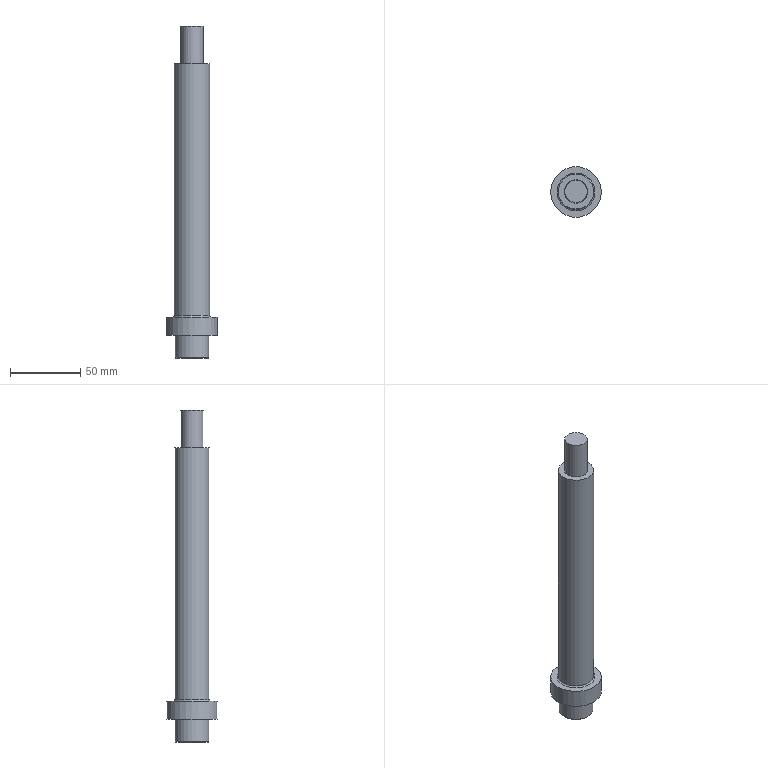Part | STEP file | 1_id4426_x_t | 1 solid | 29 faces | box 36 x 36 x 236 mm | volume 108861 mm3 | plane 18 | cylinder 6 | cone 4 | torus 1 | commonest cylinder face diameters 16.8 x2 16 x1 24 x1 25 x1 36 x1
STEP:
#1=CARTESIAN_POINT('',(3365.5,-139.,-212.));
#2=VERTEX_POINT('',#1);
#3=CARTESIAN_POINT('',(3379.,-139.,-212.));
#4=DIRECTION('',(0.,0.,1.));
#5=DIRECTION('',(-1.,0.,0.));
#6=AXIS2_PLACEMENT_3D('',#3,#4,#5);
#7=CIRCLE('',#6,13.5);
#8=EDGE_CURVE('',#2,#2,#7,.T.);
#9=ORIENTED_EDGE('',*,*,#8,.T.);
#10=EDGE_LOOP('',(#9));
#11=FACE_BOUND('',#10,.T.);
#12=CARTESIAN_POINT('',(3366.5,-139.,-211.));
#13=VERTEX_POINT('',#12);
#14=CARTESIAN_POINT('',(3379.,-139.,-211.));
#15=DIRECTION('',(0.,0.,-1.));
#16=DIRECTION('',(-1.,0.,0.));
#17=AXIS2_PLACEMENT_3D('',#14,#15,#16);
#18=CIRCLE('',#17,12.5);
#19=EDGE_CURVE('',#13,#13,#18,.T.);
#20=ORIENTED_EDGE('',*,*,#19,.T.);
#21=EDGE_LOOP('',(#20));
#22=FACE_BOUND('',#21,.T.);
#23=CARTESIAN_POINT('',(3379.,-139.,-211.));
#24=DIRECTION('',(0.,0.,-1.));
#25=DIRECTION('',(1.,0.,0.));
#26=AXIS2_PLACEMENT_3D('',#23,#24,#25);
#27=TOROIDAL_SURFACE('',#26,13.5,1.);
#28=ADVANCED_FACE('',(#11,#22),#27,.F.);
#29=CARTESIAN_POINT('',(3397.,-139.,-225.));
#30=VERTEX_POINT('',#29);
#31=CARTESIAN_POINT('',(3379.,-139.,-225.));
#32=DIRECTION('',(0.,0.,-1.));
#33=DIRECTION('',(1.,0.,0.));
#34=AXIS2_PLACEMENT_3D('',#31,#32,#33);
#35=CIRCLE('',#34,18.);
#36=EDGE_CURVE('',#30,#30,#35,.T.);
#37=ORIENTED_EDGE('',*,*,#36,.F.);
#38=EDGE_LOOP('',(#37));
#39=FACE_BOUND('',#38,.T.);
#40=CARTESIAN_POINT('',(3397.,-139.,-212.));
#41=VERTEX_POINT('',#40);
#42=CARTESIAN_POINT('',(3379.,-139.,-212.));
#43=DIRECTION('',(0.,0.,1.));
#44=DIRECTION('',(1.,0.,0.));
#45=AXIS2_PLACEMENT_3D('',#42,#43,#44);
#46=CIRCLE('',#45,18.);
#47=EDGE_CURVE('',#41,#41,#46,.T.);
#48=ORIENTED_EDGE('',*,*,#47,.F.);
#49=EDGE_LOOP('',(#48));
#50=FACE_BOUND('',#49,.T.);
#51=CARTESIAN_POINT('',(3379.,-139.,-218.5));
#52=DIRECTION('',(0.,0.,1.));
#53=DIRECTION('',(-1.,0.,0.));
#54=AXIS2_PLACEMENT_3D('',#51,#52,#53);
#55=CYLINDRICAL_SURFACE('',#54,18.);
#56=ADVANCED_FACE('',(#39,#50),#55,.T.);
#57=CARTESIAN_POINT('',(3387.4,-139.,-32.));
#58=VERTEX_POINT('',#57);
#59=CARTESIAN_POINT('',(3387.4,-139.,-225.));
#60=VERTEX_POINT('',#59);
#61=CARTESIAN_POINT('',(3387.4,-139.,-168.5));
#62=DIRECTION('',(0.,0.,-1.));
#63=VECTOR('',#62,1.);
#64=LINE('',#61,#63);
#65=EDGE_CURVE('',#58,#60,#64,.T.);
#66=ORIENTED_EDGE('',*,*,#65,.F.);
#67=CARTESIAN_POINT('',(3370.6,-139.,-32.));
#68=VERTEX_POINT('',#67);
#69=CARTESIAN_POINT('',(3379.,-139.,-32.));
#70=DIRECTION('',(0.,0.,-1.));
#71=DIRECTION('',(1.,0.,0.));
#72=AXIS2_PLACEMENT_3D('',#69,#70,#71);
#73=CIRCLE('',#72,8.4);
#74=EDGE_CURVE('',#68,#58,#73,.T.);
#75=ORIENTED_EDGE('',*,*,#74,.F.);
#76=CARTESIAN_POINT('',(3370.6,-139.,-225.));
#77=VERTEX_POINT('',#76);
#78=CARTESIAN_POINT('',(3370.6,-139.,-168.5));
#79=DIRECTION('',(0.,0.,1.));
#80=VECTOR('',#79,1.);
#81=LINE('',#78,#80);
#82=EDGE_CURVE('',#77,#68,#81,.T.);
#83=ORIENTED_EDGE('',*,*,#82,.F.);
#84=CARTESIAN_POINT('',(3379.,-139.,-225.));
#85=DIRECTION('',(0.,0.,1.));
#86=DIRECTION('',(1.,0.,0.));
#87=AXIS2_PLACEMENT_3D('',#84,#85,#86);
#88=CIRCLE('',#87,8.4);
#89=EDGE_CURVE('',#60,#77,#88,.T.);
#90=ORIENTED_EDGE('',*,*,#89,.F.);
#91=EDGE_LOOP('',(#66,#75,#83,#90));
#92=FACE_OUTER_BOUND('',#91,.T.);
#93=CARTESIAN_POINT('',(3379.,-139.,-168.5));
#94=DIRECTION('',(0.,0.,1.));
#95=DIRECTION('',(-1.,0.,0.));
#96=AXIS2_PLACEMENT_3D('',#93,#94,#95);
#97=CYLINDRICAL_SURFACE('',#96,8.4);
#98=ADVANCED_FACE('',(#92),#97,.F.);
#99=ORIENTED_EDGE('',*,*,#19,.F.);
#100=EDGE_LOOP('',(#99));
#101=FACE_BOUND('',#100,.T.);
#102=CARTESIAN_POINT('',(3391.5,-139.,-32.));
#103=VERTEX_POINT('',#102);
#104=CARTESIAN_POINT('',(3379.,-139.,-32.));
#105=DIRECTION('',(0.,0.,1.));
#106=DIRECTION('',(1.,0.,0.));
#107=AXIS2_PLACEMENT_3D('',#104,#105,#106);
#108=CIRCLE('',#107,12.5);
#109=EDGE_CURVE('',#103,#103,#108,.T.);
#110=ORIENTED_EDGE('',*,*,#109,.F.);
#111=EDGE_LOOP('',(#110));
#112=FACE_BOUND('',#111,.T.);
#113=CARTESIAN_POINT('',(3379.,-139.,-162.));
#114=DIRECTION('',(0.,0.,1.));
#115=DIRECTION('',(-1.,0.,0.));
#116=AXIS2_PLACEMENT_3D('',#113,#114,#115);
#117=CYLINDRICAL_SURFACE('',#116,12.5);
#118=ADVANCED_FACE('',(#101,#112),#117,.T.);
#119=CARTESIAN_POINT('',(3387.,-139.,-225.));
#120=VERTEX_POINT('',#119);
#121=CARTESIAN_POINT('',(3379.,-139.,-225.));
#122=DIRECTION('',(0.,0.,-1.));
#123=DIRECTION('',(1.,0.,0.));
#124=AXIS2_PLACEMENT_3D('',#121,#122,#123);
#125=CIRCLE('',#124,8.);
#126=EDGE_CURVE('',#120,#120,#125,.T.);
#127=ORIENTED_EDGE('',*,*,#126,.F.);
#128=EDGE_LOOP('',(#127));
#129=FACE_BOUND('',#128,.T.);
#130=CARTESIAN_POINT('',(3387.,-139.,-5.));
#131=VERTEX_POINT('',#130);
#132=CARTESIAN_POINT('',(3379.,-139.,-5.));
#133=DIRECTION('',(0.,0.,1.));
#134=DIRECTION('',(1.,0.,0.));
#135=AXIS2_PLACEMENT_3D('',#132,#133,#134);
#136=CIRCLE('',#135,8.);
#137=EDGE_CURVE('',#131,#131,#136,.T.);
#138=ORIENTED_EDGE('',*,*,#137,.F.);
#139=EDGE_LOOP('',(#138));
#140=FACE_BOUND('',#139,.T.);
#141=CARTESIAN_POINT('',(3379.,-139.,-155.));
#142=DIRECTION('',(0.,0.,1.));
#143=DIRECTION('',(-1.,0.,0.));
#144=AXIS2_PLACEMENT_3D('',#141,#142,#143);
#145=CYLINDRICAL_SURFACE('',#144,8.);
#146=ADVANCED_FACE('',(#129,#140),#145,.T.);
#147=CARTESIAN_POINT('',(3370.917,-139.,-233.));
#148=VERTEX_POINT('',#147);
#149=CARTESIAN_POINT('',(3379.,-139.,-232.));
#150=VERTEX_POINT('',#149);
#151=CARTESIAN_POINT('',(3374.959,-139.,-232.5));
#152=DIRECTION('',(0.9924,0.,0.1228));
#153=VECTOR('',#152,1.);
#154=LINE('',#151,#153);
#155=EDGE_CURVE('',#148,#150,#154,.T.);
#156=ORIENTED_EDGE('',*,*,#155,.T.);
#157=CARTESIAN_POINT('',(3387.083,-139.,-233.));
#158=VERTEX_POINT('',#157);
#159=CARTESIAN_POINT('',(3383.041,-139.,-232.5));
#160=DIRECTION('',(0.9924,0.,-0.1228));
#161=VECTOR('',#160,1.);
#162=LINE('',#159,#161);
#163=EDGE_CURVE('',#150,#158,#162,.T.);
#164=ORIENTED_EDGE('',*,*,#163,.T.);
#165=CARTESIAN_POINT('',(3386.,-143.041,-233.));
#166=VERTEX_POINT('',#165);
#167=CARTESIAN_POINT('',(3379.,-139.,-233.));
#168=DIRECTION('',(0.,0.,-1.));
#169=DIRECTION('',(1.,0.,0.));
#170=AXIS2_PLACEMENT_3D('',#167,#168,#169);
#171=CIRCLE('',#170,8.083);
#172=EDGE_CURVE('',#158,#166,#171,.T.);
#173=ORIENTED_EDGE('',*,*,#172,.T.);
#174=CARTESIAN_POINT('',(3379.,-147.083,-233.));
#175=VERTEX_POINT('',#174);
#176=CARTESIAN_POINT('',(3379.,-139.,-233.));
#177=DIRECTION('',(0.,0.,-1.));
#178=DIRECTION('',(1.,0.,0.));
#179=AXIS2_PLACEMENT_3D('',#176,#177,#178);
#180=CIRCLE('',#179,8.083);
#181=EDGE_CURVE('',#166,#175,#180,.T.);
#182=ORIENTED_EDGE('',*,*,#181,.T.);
#183=CARTESIAN_POINT('',(3372.,-143.041,-233.));
#184=VERTEX_POINT('',#183);
#185=CARTESIAN_POINT('',(3379.,-139.,-233.));
#186=DIRECTION('',(0.,0.,-1.));
#187=DIRECTION('',(1.,0.,0.));
#188=AXIS2_PLACEMENT_3D('',#185,#186,#187);
#189=CIRCLE('',#188,8.083);
#190=EDGE_CURVE('',#175,#184,#189,.T.);
#191=ORIENTED_EDGE('',*,*,#190,.T.);
#192=CARTESIAN_POINT('',(3379.,-139.,-233.));
#193=DIRECTION('',(0.,0.,-1.));
#194=DIRECTION('',(1.,0.,0.));
#195=AXIS2_PLACEMENT_3D('',#192,#193,#194);
#196=CIRCLE('',#195,8.083);
#197=EDGE_CURVE('',#184,#148,#196,.T.);
#198=ORIENTED_EDGE('',*,*,#197,.T.);
#199=EDGE_LOOP('',(#156,#164,#173,#182,#191,#198));
#200=FACE_OUTER_BOUND('',#199,.T.);
#201=CARTESIAN_POINT('',(3379.,-139.,-232.5));
#202=DIRECTION('',(0.,0.,-1.));
#203=DIRECTION('',(-1.,0.,0.));
#204=AXIS2_PLACEMENT_3D('',#201,#202,#203);
#205=CONICAL_SURFACE('',#204,4.041,82.947);
#206=ADVANCED_FACE('',(#200),#205,.F.);
#207=CARTESIAN_POINT('',(3391.,-139.,-240.5));
#208=VERTEX_POINT('',#207);
#209=CARTESIAN_POINT('',(3367.,-139.,-240.5));
#210=VERTEX_POINT('',#209);
#211=CARTESIAN_POINT('',(3379.,-139.,-240.5));
#212=DIRECTION('',(0.,0.,-1.));
#213=DIRECTION('',(-1.,0.,0.));
#214=AXIS2_PLACEMENT_3D('',#211,#212,#213);
#215=CIRCLE('',#214,12.);
#216=EDGE_CURVE('',#208,#210,#215,.T.);
#217=ORIENTED_EDGE('',*,*,#216,.F.);
#218=CARTESIAN_POINT('',(3379.,-139.,-240.5));
#219=DIRECTION('',(0.,0.,-1.));
#220=DIRECTION('',(-1.,0.,0.));
#221=AXIS2_PLACEMENT_3D('',#218,#219,#220);
#222=CIRCLE('',#221,12.);
#223=EDGE_CURVE('',#210,#208,#222,.T.);
#224=ORIENTED_EDGE('',*,*,#223,.F.);
#225=EDGE_LOOP('',(#217,#224));
#226=FACE_BOUND('',#225,.T.);
#227=CARTESIAN_POINT('',(3391.,-139.,-225.));
#228=VERTEX_POINT('',#227);
#229=CARTESIAN_POINT('',(3379.,-139.,-225.));
#230=DIRECTION('',(0.,0.,1.));
#231=DIRECTION('',(1.,0.,0.));
#232=AXIS2_PLACEMENT_3D('',#229,#230,#231);
#233=CIRCLE('',#232,12.);
#234=EDGE_CURVE('',#228,#228,#233,.T.);
#235=ORIENTED_EDGE('',*,*,#234,.F.);
#236=EDGE_LOOP('',(#235));
#237=FACE_BOUND('',#236,.T.);
#238=CARTESIAN_POINT('',(3379.,-139.,-233.));
#239=DIRECTION('',(0.,0.,1.));
#240=DIRECTION('',(-1.,0.,0.));
#241=AXIS2_PLACEMENT_3D('',#238,#239,#240);
#242=CYLINDRICAL_SURFACE('',#241,12.);
#243=ADVANCED_FACE('',(#226,#237),#242,.T.);
#244=CARTESIAN_POINT('',(3367.5,-139.,-241.));
#245=VERTEX_POINT('',#244);
#246=CARTESIAN_POINT('',(3367.5,-139.,-241.));
#247=DIRECTION('',(0.7071,0.,-0.7071));
#248=VECTOR('',#247,1.);
#249=LINE('',#246,#248);
#250=EDGE_CURVE('',#210,#245,#249,.T.);
#251=ORIENTED_EDGE('',*,*,#250,.F.);
#252=ORIENTED_EDGE('',*,*,#223,.T.);
#253=CARTESIAN_POINT('',(3390.5,-139.,-241.));
#254=VERTEX_POINT('',#253);
#255=CARTESIAN_POINT('',(3390.5,-139.,-241.));
#256=DIRECTION('',(0.7071,0.,0.7071));
#257=VECTOR('',#256,1.);
#258=LINE('',#255,#257);
#259=EDGE_CURVE('',#254,#208,#258,.T.);
#260=ORIENTED_EDGE('',*,*,#259,.F.);
#261=CARTESIAN_POINT('',(3379.,-139.,-241.));
#262=DIRECTION('',(0.,0.,1.));
#263=DIRECTION('',(-1.,0.,0.));
#264=AXIS2_PLACEMENT_3D('',#261,#262,#263);
#265=CIRCLE('',#264,11.5);
#266=EDGE_CURVE('',#254,#245,#265,.T.);
#267=ORIENTED_EDGE('',*,*,#266,.T.);
#268=EDGE_LOOP('',(#251,#252,#260,#267));
#269=FACE_OUTER_BOUND('',#268,.T.);
#270=CARTESIAN_POINT('',(3379.,-139.,-241.));
#271=DIRECTION('',(0.,0.,1.));
#272=DIRECTION('',(1.,0.,0.));
#273=AXIS2_PLACEMENT_3D('',#270,#271,#272);
#274=CONICAL_SURFACE('',#273,11.5,45.);
#275=ADVANCED_FACE('',(#269),#274,.T.);
#276=ORIENTED_EDGE('',*,*,#126,.T.);
#277=EDGE_LOOP('',(#276));
#278=FACE_BOUND('',#277,.T.);
#279=ORIENTED_EDGE('',*,*,#89,.T.);
#280=CARTESIAN_POINT('',(3379.,-139.,-225.));
#281=DIRECTION('',(0.,0.,1.));
#282=DIRECTION('',(1.,0.,0.));
#283=AXIS2_PLACEMENT_3D('',#280,#281,#282);
#284=CIRCLE('',#283,8.4);
#285=EDGE_CURVE('',#77,#60,#284,.T.);
#286=ORIENTED_EDGE('',*,*,#285,.T.);
#287=EDGE_LOOP('',(#279,#286));
#288=FACE_BOUND('',#287,.T.);
#289=CARTESIAN_POINT('',(3379.,-139.,-225.));
#290=DIRECTION('',(0.,0.,1.));
#291=DIRECTION('',(-1.,0.,0.));
#292=AXIS2_PLACEMENT_3D('',#289,#290,#291);
#293=PLANE('',#292);
#294=ADVANCED_FACE('',(#278,#288),#293,.T.);
#295=ORIENTED_EDGE('',*,*,#250,.T.);
#296=CARTESIAN_POINT('',(3379.,-139.,-241.));
#297=DIRECTION('',(0.,0.,1.));
#298=DIRECTION('',(-1.,0.,0.));
#299=AXIS2_PLACEMENT_3D('',#296,#297,#298);
#300=CIRCLE('',#299,11.5);
#301=EDGE_CURVE('',#245,#254,#300,.T.);
#302=ORIENTED_EDGE('',*,*,#301,.T.);
#303=ORIENTED_EDGE('',*,*,#259,.T.);
#304=ORIENTED_EDGE('',*,*,#216,.T.);
#305=EDGE_LOOP('',(#295,#302,#303,#304));
#306=FACE_OUTER_BOUND('',#305,.T.);
#307=CARTESIAN_POINT('',(3379.,-139.,-241.));
#308=DIRECTION('',(0.,0.,1.));
#309=DIRECTION('',(1.,0.,0.));
#310=AXIS2_PLACEMENT_3D('',#307,#308,#309);
#311=CONICAL_SURFACE('',#310,11.5,45.);
#312=ADVANCED_FACE('',(#306),#311,.T.);
#313=CARTESIAN_POINT('',(3379.,-147.083,-241.));
#314=VERTEX_POINT('',#313);
#315=CARTESIAN_POINT('',(3386.,-143.041,-241.));
#316=VERTEX_POINT('',#315);
#317=CARTESIAN_POINT('',(3382.5,-145.062,-241.));
#318=DIRECTION('',(0.866,0.5,0.));
#319=VECTOR('',#318,1.);
#320=LINE('',#317,#319);
#321=EDGE_CURVE('',#314,#316,#320,.T.);
#322=ORIENTED_EDGE('',*,*,#321,.T.);
#323=CARTESIAN_POINT('',(3386.,-134.958,-241.));
#324=VERTEX_POINT('',#323);
#325=CARTESIAN_POINT('',(3386.,-139.,-241.));
#326=DIRECTION('',(0.,1.,0.));
#327=VECTOR('',#326,1.);
#328=LINE('',#325,#327);
#329=EDGE_CURVE('',#316,#324,#328,.T.);
#330=ORIENTED_EDGE('',*,*,#329,.T.);
#331=CARTESIAN_POINT('',(3379.,-130.917,-241.));
#332=VERTEX_POINT('',#331);
#333=CARTESIAN_POINT('',(3382.5,-132.938,-241.));
#334=DIRECTION('',(-0.866,0.5,0.));
#335=VECTOR('',#334,1.);
#336=LINE('',#333,#335);
#337=EDGE_CURVE('',#324,#332,#336,.T.);
#338=ORIENTED_EDGE('',*,*,#337,.T.);
#339=CARTESIAN_POINT('',(3372.,-134.958,-241.));
#340=VERTEX_POINT('',#339);
#341=CARTESIAN_POINT('',(3375.5,-132.938,-241.));
#342=DIRECTION('',(-0.866,-0.5,0.));
#343=VECTOR('',#342,1.);
#344=LINE('',#341,#343);
#345=EDGE_CURVE('',#332,#340,#344,.T.);
#346=ORIENTED_EDGE('',*,*,#345,.T.);
#347=CARTESIAN_POINT('',(3372.,-143.041,-241.));
#348=VERTEX_POINT('',#347);
#349=CARTESIAN_POINT('',(3372.,-139.,-241.));
#350=DIRECTION('',(0.,-1.,0.));
#351=VECTOR('',#350,1.);
#352=LINE('',#349,#351);
#353=EDGE_CURVE('',#340,#348,#352,.T.);
#354=ORIENTED_EDGE('',*,*,#353,.T.);
#355=CARTESIAN_POINT('',(3375.5,-145.062,-241.));
#356=DIRECTION('',(0.866,-0.5,0.));
#357=VECTOR('',#356,1.);
#358=LINE('',#355,#357);
#359=EDGE_CURVE('',#348,#314,#358,.T.);
#360=ORIENTED_EDGE('',*,*,#359,.T.);
#361=EDGE_LOOP('',(#322,#330,#338,#346,#354,#360));
#362=FACE_BOUND('',#361,.T.);
#363=ORIENTED_EDGE('',*,*,#266,.F.);
#364=ORIENTED_EDGE('',*,*,#301,.F.);
#365=EDGE_LOOP('',(#363,#364));
#366=FACE_BOUND('',#365,.T.);
#367=CARTESIAN_POINT('',(3379.,-139.,-241.));
#368=DIRECTION('',(0.,0.,-1.));
#369=DIRECTION('',(1.,0.,0.));
#370=AXIS2_PLACEMENT_3D('',#367,#368,#369);
#371=PLANE('',#370);
#372=ADVANCED_FACE('',(#362,#366),#371,.T.);
#373=CARTESIAN_POINT('',(3382.5,-145.062,-233.));
#374=DIRECTION('',(0.866,0.5,0.));
#375=VECTOR('',#374,1.);
#376=LINE('',#373,#375);
#377=EDGE_CURVE('',#175,#166,#376,.T.);
#378=ORIENTED_EDGE('',*,*,#377,.F.);
#379=ORIENTED_EDGE('',*,*,#181,.F.);
#380=EDGE_LOOP('',(#378,#379));
#381=FACE_OUTER_BOUND('',#380,.T.);
#382=CARTESIAN_POINT('',(3379.,-139.,-233.));
#383=DIRECTION('',(0.,0.,-1.));
#384=DIRECTION('',(1.,0.,0.));
#385=AXIS2_PLACEMENT_3D('',#382,#383,#384);
#386=PLANE('',#385);
#387=ADVANCED_FACE('',(#381),#386,.F.);
#388=CARTESIAN_POINT('',(3386.,-134.958,-233.));
#389=VERTEX_POINT('',#388);
#390=CARTESIAN_POINT('',(3386.,-139.,-233.));
#391=DIRECTION('',(0.,1.,0.));
#392=VECTOR('',#391,1.);
#393=LINE('',#390,#392);
#394=EDGE_CURVE('',#166,#389,#393,.T.);
#395=ORIENTED_EDGE('',*,*,#394,.F.);
#396=ORIENTED_EDGE('',*,*,#172,.F.);
#397=CARTESIAN_POINT('',(3379.,-139.,-233.));
#398=DIRECTION('',(0.,0.,-1.));
#399=DIRECTION('',(1.,0.,0.));
#400=AXIS2_PLACEMENT_3D('',#397,#398,#399);
#401=CIRCLE('',#400,8.083);
#402=EDGE_CURVE('',#389,#158,#401,.T.);
#403=ORIENTED_EDGE('',*,*,#402,.F.);
#404=EDGE_LOOP('',(#395,#396,#403));
#405=FACE_OUTER_BOUND('',#404,.T.);
#406=CARTESIAN_POINT('',(3379.,-139.,-233.));
#407=DIRECTION('',(0.,0.,-1.));
#408=DIRECTION('',(1.,0.,0.));
#409=AXIS2_PLACEMENT_3D('',#406,#407,#408);
#410=PLANE('',#409);
#411=ADVANCED_FACE('',(#405),#410,.F.);
#412=CARTESIAN_POINT('',(3379.,-130.917,-233.));
#413=VERTEX_POINT('',#412);
#414=CARTESIAN_POINT('',(3382.5,-132.938,-233.));
#415=DIRECTION('',(-0.866,0.5,0.));
#416=VECTOR('',#415,1.);
#417=LINE('',#414,#416);
#418=EDGE_CURVE('',#389,#413,#417,.T.);
#419=ORIENTED_EDGE('',*,*,#418,.F.);
#420=CARTESIAN_POINT('',(3379.,-139.,-233.));
#421=DIRECTION('',(0.,0.,-1.));
#422=DIRECTION('',(1.,0.,0.));
#423=AXIS2_PLACEMENT_3D('',#420,#421,#422);
#424=CIRCLE('',#423,8.083);
#425=EDGE_CURVE('',#413,#389,#424,.T.);
#426=ORIENTED_EDGE('',*,*,#425,.F.);
#427=EDGE_LOOP('',(#419,#426));
#428=FACE_OUTER_BOUND('',#427,.T.);
#429=CARTESIAN_POINT('',(3379.,-139.,-233.));
#430=DIRECTION('',(0.,0.,-1.));
#431=DIRECTION('',(1.,0.,0.));
#432=AXIS2_PLACEMENT_3D('',#429,#430,#431);
#433=PLANE('',#432);
#434=ADVANCED_FACE('',(#428),#433,.F.);
#435=CARTESIAN_POINT('',(3372.,-134.958,-233.));
#436=VERTEX_POINT('',#435);
#437=CARTESIAN_POINT('',(3375.5,-132.938,-233.));
#438=DIRECTION('',(-0.866,-0.5,0.));
#439=VECTOR('',#438,1.);
#440=LINE('',#437,#439);
#441=EDGE_CURVE('',#413,#436,#440,.T.);
#442=ORIENTED_EDGE('',*,*,#441,.F.);
#443=CARTESIAN_POINT('',(3379.,-139.,-233.));
#444=DIRECTION('',(0.,0.,-1.));
#445=DIRECTION('',(1.,0.,0.));
#446=AXIS2_PLACEMENT_3D('',#443,#444,#445);
#447=CIRCLE('',#446,8.083);
#448=EDGE_CURVE('',#436,#413,#447,.T.);
#449=ORIENTED_EDGE('',*,*,#448,.F.);
#450=EDGE_LOOP('',(#442,#449));
#451=FACE_OUTER_BOUND('',#450,.T.);
#452=CARTESIAN_POINT('',(3379.,-139.,-233.));
#453=DIRECTION('',(0.,0.,-1.));
#454=DIRECTION('',(1.,0.,0.));
#455=AXIS2_PLACEMENT_3D('',#452,#453,#454);
#456=PLANE('',#455);
#457=ADVANCED_FACE('',(#451),#456,.F.);
#458=CARTESIAN_POINT('',(3372.,-139.,-233.));
#459=DIRECTION('',(0.,-1.,0.));
#460=VECTOR('',#459,1.);
#461=LINE('',#458,#460);
#462=EDGE_CURVE('',#436,#184,#461,.T.);
#463=ORIENTED_EDGE('',*,*,#462,.F.);
#464=CARTESIAN_POINT('',(3379.,-139.,-233.));
#465=DIRECTION('',(0.,0.,-1.));
#466=DIRECTION('',(1.,0.,0.));
#467=AXIS2_PLACEMENT_3D('',#464,#465,#466);
#468=CIRCLE('',#467,8.083);
#469=EDGE_CURVE('',#148,#436,#468,.T.);
#470=ORIENTED_EDGE('',*,*,#469,.F.);
#471=ORIENTED_EDGE('',*,*,#197,.F.);
#472=EDGE_LOOP('',(#463,#470,#471));
#473=FACE_OUTER_BOUND('',#472,.T.);
#474=CARTESIAN_POINT('',(3379.,-139.,-233.));
#475=DIRECTION('',(0.,0.,-1.));
#476=DIRECTION('',(1.,0.,0.));
#477=AXIS2_PLACEMENT_3D('',#474,#475,#476);
#478=PLANE('',#477);
#479=ADVANCED_FACE('',(#473),#478,.F.);
#480=CARTESIAN_POINT('',(3375.5,-145.062,-233.));
#481=DIRECTION('',(0.866,-0.5,0.));
#482=VECTOR('',#481,1.);
#483=LINE('',#480,#482);
#484=EDGE_CURVE('',#184,#175,#483,.T.);
#485=ORIENTED_EDGE('',*,*,#484,.F.);
#486=ORIENTED_EDGE('',*,*,#190,.F.);
#487=EDGE_LOOP('',(#485,#486));
#488=FACE_OUTER_BOUND('',#487,.T.);
#489=CARTESIAN_POINT('',(3379.,-139.,-233.));
#490=DIRECTION('',(0.,0.,-1.));
#491=DIRECTION('',(1.,0.,0.));
#492=AXIS2_PLACEMENT_3D('',#489,#490,#491);
#493=PLANE('',#492);
#494=ADVANCED_FACE('',(#488),#493,.F.);
#495=ORIENTED_EDGE('',*,*,#155,.F.);
#496=ORIENTED_EDGE('',*,*,#469,.T.);
#497=ORIENTED_EDGE('',*,*,#448,.T.);
#498=ORIENTED_EDGE('',*,*,#425,.T.);
#499=ORIENTED_EDGE('',*,*,#402,.T.);
#500=ORIENTED_EDGE('',*,*,#163,.F.);
#501=EDGE_LOOP('',(#495,#496,#497,#498,#499,#500));
#502=FACE_OUTER_BOUND('',#501,.T.);
#503=CARTESIAN_POINT('',(3379.,-139.,-232.5));
#504=DIRECTION('',(0.,0.,-1.));
#505=DIRECTION('',(-1.,0.,0.));
#506=AXIS2_PLACEMENT_3D('',#503,#504,#505);
#507=CONICAL_SURFACE('',#506,4.041,82.947);
#508=ADVANCED_FACE('',(#502),#507,.F.);
#509=CARTESIAN_POINT('',(3379.,-147.083,-237.));
#510=DIRECTION('',(0.,0.,-1.));
#511=VECTOR('',#510,1.);
#512=LINE('',#509,#511);
#513=EDGE_CURVE('',#175,#314,#512,.T.);
#514=ORIENTED_EDGE('',*,*,#513,.F.);
#515=ORIENTED_EDGE('',*,*,#377,.T.);
#516=CARTESIAN_POINT('',(3386.,-143.041,-237.));
#517=DIRECTION('',(0.,0.,-1.));
#518=VECTOR('',#517,1.);
#519=LINE('',#516,#518);
#520=EDGE_CURVE('',#166,#316,#519,.T.);
#521=ORIENTED_EDGE('',*,*,#520,.T.);
#522=ORIENTED_EDGE('',*,*,#321,.F.);
#523=EDGE_LOOP('',(#514,#515,#521,#522));
#524=FACE_OUTER_BOUND('',#523,.T.);
#525=CARTESIAN_POINT('',(3382.5,-145.062,-237.));
#526=DIRECTION('',(-0.5,0.866,0.));
#527=DIRECTION('',(0.,0.,-1.));
#528=AXIS2_PLACEMENT_3D('',#525,#526,#527);
#529=PLANE('',#528);
#530=ADVANCED_FACE('',(#524),#529,.T.);
#531=CARTESIAN_POINT('',(3372.,-143.041,-237.));
#532=DIRECTION('',(0.,0.,-1.));
#533=VECTOR('',#532,1.);
#534=LINE('',#531,#533);
#535=EDGE_CURVE('',#184,#348,#534,.T.);
#536=ORIENTED_EDGE('',*,*,#535,.F.);
#537=ORIENTED_EDGE('',*,*,#484,.T.);
#538=ORIENTED_EDGE('',*,*,#513,.T.);
#539=ORIENTED_EDGE('',*,*,#359,.F.);
#540=EDGE_LOOP('',(#536,#537,#538,#539));
#541=FACE_OUTER_BOUND('',#540,.T.);
#542=CARTESIAN_POINT('',(3375.5,-145.062,-237.));
#543=DIRECTION('',(0.5,0.866,0.));
#544=DIRECTION('',(0.,0.,1.));
#545=AXIS2_PLACEMENT_3D('',#542,#543,#544);
#546=PLANE('',#545);
#547=ADVANCED_FACE('',(#541),#546,.T.);
#548=CARTESIAN_POINT('',(3372.,-134.958,-237.));
#549=DIRECTION('',(0.,0.,-1.));
#550=VECTOR('',#549,1.);
#551=LINE('',#548,#550);
#552=EDGE_CURVE('',#436,#340,#551,.T.);
#553=ORIENTED_EDGE('',*,*,#552,.F.);
#554=ORIENTED_EDGE('',*,*,#462,.T.);
#555=ORIENTED_EDGE('',*,*,#535,.T.);
#556=ORIENTED_EDGE('',*,*,#353,.F.);
#557=EDGE_LOOP('',(#553,#554,#555,#556));
#558=FACE_OUTER_BOUND('',#557,.T.);
#559=CARTESIAN_POINT('',(3372.,-139.,-237.));
#560=DIRECTION('',(1.,0.,0.));
#561=DIRECTION('',(0.,0.,1.));
#562=AXIS2_PLACEMENT_3D('',#559,#560,#561);
#563=PLANE('',#562);
#564=ADVANCED_FACE('',(#558),#563,.T.);
#565=CARTESIAN_POINT('',(3379.,-130.917,-237.));
#566=DIRECTION('',(0.,0.,-1.));
#567=VECTOR('',#566,1.);
#568=LINE('',#565,#567);
#569=EDGE_CURVE('',#413,#332,#568,.T.);
#570=ORIENTED_EDGE('',*,*,#569,.F.);
#571=ORIENTED_EDGE('',*,*,#441,.T.);
#572=ORIENTED_EDGE('',*,*,#552,.T.);
#573=ORIENTED_EDGE('',*,*,#345,.F.);
#574=EDGE_LOOP('',(#570,#571,#572,#573));
#575=FACE_OUTER_BOUND('',#574,.T.);
#576=CARTESIAN_POINT('',(3375.5,-132.938,-237.));
#577=DIRECTION('',(0.5,-0.866,0.));
#578=DIRECTION('',(0.,0.,1.));
#579=AXIS2_PLACEMENT_3D('',#576,#577,#578);
#580=PLANE('',#579);
#581=ADVANCED_FACE('',(#575),#580,.T.);
#582=CARTESIAN_POINT('',(3386.,-134.958,-237.));
#583=DIRECTION('',(0.,0.,-1.));
#584=VECTOR('',#583,1.);
#585=LINE('',#582,#584);
#586=EDGE_CURVE('',#389,#324,#585,.T.);
#587=ORIENTED_EDGE('',*,*,#586,.F.);
#588=ORIENTED_EDGE('',*,*,#418,.T.);
#589=ORIENTED_EDGE('',*,*,#569,.T.);
#590=ORIENTED_EDGE('',*,*,#337,.F.);
#591=EDGE_LOOP('',(#587,#588,#589,#590));
#592=FACE_OUTER_BOUND('',#591,.T.);
#593=CARTESIAN_POINT('',(3382.5,-132.938,-237.));
#594=DIRECTION('',(-0.5,-0.866,0.));
#595=DIRECTION('',(0.,0.,-1.));
#596=AXIS2_PLACEMENT_3D('',#593,#594,#595);
#597=PLANE('',#596);
#598=ADVANCED_FACE('',(#592),#597,.T.);
#599=ORIENTED_EDGE('',*,*,#520,.F.);
#600=ORIENTED_EDGE('',*,*,#394,.T.);
#601=ORIENTED_EDGE('',*,*,#586,.T.);
#602=ORIENTED_EDGE('',*,*,#329,.F.);
#603=EDGE_LOOP('',(#599,#600,#601,#602));
#604=FACE_OUTER_BOUND('',#603,.T.);
#605=CARTESIAN_POINT('',(3386.,-139.,-237.));
#606=DIRECTION('',(-1.,0.,0.));
#607=DIRECTION('',(0.,0.,-1.));
#608=AXIS2_PLACEMENT_3D('',#605,#606,#607);
#609=PLANE('',#608);
#610=ADVANCED_FACE('',(#604),#609,.T.);
#611=ORIENTED_EDGE('',*,*,#137,.T.);
#612=EDGE_LOOP('',(#611));
#613=FACE_OUTER_BOUND('',#612,.T.);
#614=CARTESIAN_POINT('',(3379.,-139.,-5.));
#615=DIRECTION('',(0.,0.,1.));
#616=DIRECTION('',(-1.,0.,0.));
#617=AXIS2_PLACEMENT_3D('',#614,#615,#616);
#618=PLANE('',#617);
#619=ADVANCED_FACE('',(#613),#618,.T.);
#620=ORIENTED_EDGE('',*,*,#47,.T.);
#621=EDGE_LOOP('',(#620));
#622=FACE_BOUND('',#621,.T.);
#623=ORIENTED_EDGE('',*,*,#8,.F.);
#624=EDGE_LOOP('',(#623));
#625=FACE_BOUND('',#624,.T.);
#626=CARTESIAN_POINT('',(3379.,-139.,-212.));
#627=DIRECTION('',(0.,0.,1.));
#628=DIRECTION('',(-1.,0.,0.));
#629=AXIS2_PLACEMENT_3D('',#626,#627,#628);
#630=PLANE('',#629);
#631=ADVANCED_FACE('',(#622,#625),#630,.T.);
#632=ORIENTED_EDGE('',*,*,#65,.T.);
#633=ORIENTED_EDGE('',*,*,#285,.F.);
#634=ORIENTED_EDGE('',*,*,#82,.T.);
#635=CARTESIAN_POINT('',(3379.,-139.,-32.));
#636=DIRECTION('',(0.,0.,-1.));
#637=DIRECTION('',(1.,0.,0.));
#638=AXIS2_PLACEMENT_3D('',#635,#636,#637);
#639=CIRCLE('',#638,8.4);
#640=EDGE_CURVE('',#58,#68,#639,.T.);
#641=ORIENTED_EDGE('',*,*,#640,.F.);
#642=EDGE_LOOP('',(#632,#633,#634,#641));
#643=FACE_OUTER_BOUND('',#642,.T.);
#644=CARTESIAN_POINT('',(3379.,-139.,-168.5));
#645=DIRECTION('',(0.,0.,1.));
#646=DIRECTION('',(-1.,0.,0.));
#647=AXIS2_PLACEMENT_3D('',#644,#645,#646);
#648=CYLINDRICAL_SURFACE('',#647,8.4);
#649=ADVANCED_FACE('',(#643),#648,.F.);
#650=ORIENTED_EDGE('',*,*,#640,.T.);
#651=ORIENTED_EDGE('',*,*,#74,.T.);
#652=EDGE_LOOP('',(#650,#651));
#653=FACE_BOUND('',#652,.T.);
#654=ORIENTED_EDGE('',*,*,#109,.T.);
#655=EDGE_LOOP('',(#654));
#656=FACE_BOUND('',#655,.T.);
#657=CARTESIAN_POINT('',(3379.,-139.,-32.));
#658=DIRECTION('',(0.,0.,1.));
#659=DIRECTION('',(-1.,0.,0.));
#660=AXIS2_PLACEMENT_3D('',#657,#658,#659);
#661=PLANE('',#660);
#662=ADVANCED_FACE('',(#653,#656),#661,.T.);
#663=ORIENTED_EDGE('',*,*,#234,.T.);
#664=EDGE_LOOP('',(#663));
#665=FACE_BOUND('',#664,.T.);
#666=ORIENTED_EDGE('',*,*,#36,.T.);
#667=EDGE_LOOP('',(#666));
#668=FACE_BOUND('',#667,.T.);
#669=CARTESIAN_POINT('',(3379.,-139.,-225.));
#670=DIRECTION('',(0.,0.,-1.));
#671=DIRECTION('',(1.,0.,0.));
#672=AXIS2_PLACEMENT_3D('',#669,#670,#671);
#673=PLANE('',#672);
#674=ADVANCED_FACE('',(#665,#668),#673,.T.);
#675=CLOSED_SHELL('',(#28,#56,#98,#118,#146,#206,#243,#275,#294,#312,#372,#387,#411,#434,#457,#479,#494,#508,#530,#547,#564,#581,#598,#610,#619,#631,#649,#662,#674));
#676=MANIFOLD_SOLID_BREP('',#675);
#677=(LENGTH_UNIT()NAMED_UNIT(*)SI_UNIT(.MILLI.,.METRE.));
#678=UNCERTAINTY_MEASURE_WITH_UNIT(LENGTH_MEASURE(0.00002),#677,'','');
#679=(NAMED_UNIT(*)PLANE_ANGLE_UNIT()SI_UNIT($,.RADIAN.));
#680=PLANE_ANGLE_MEASURE_WITH_UNIT(PLANE_ANGLE_MEASURE(0.01745),#679);
#681=DIMENSIONAL_EXPONENTS(0.,0.,0.,0.,0.,0.,0.);
#682=(CONVERSION_BASED_UNIT('DEGREE',#680)NAMED_UNIT(#681)PLANE_ANGLE_UNIT());
#683=(NAMED_UNIT(*)SI_UNIT($,.STERADIAN.)SOLID_ANGLE_UNIT());
#684=(GEOMETRIC_REPRESENTATION_CONTEXT(3)GLOBAL_UNCERTAINTY_ASSIGNED_CONTEXT((#678))GLOBAL_UNIT_ASSIGNED_CONTEXT((#677,#682,#683))REPRESENTATION_CONTEXT('',''));
#685=ADVANCED_BREP_SHAPE_REPRESENTATION('',(#676),#684);